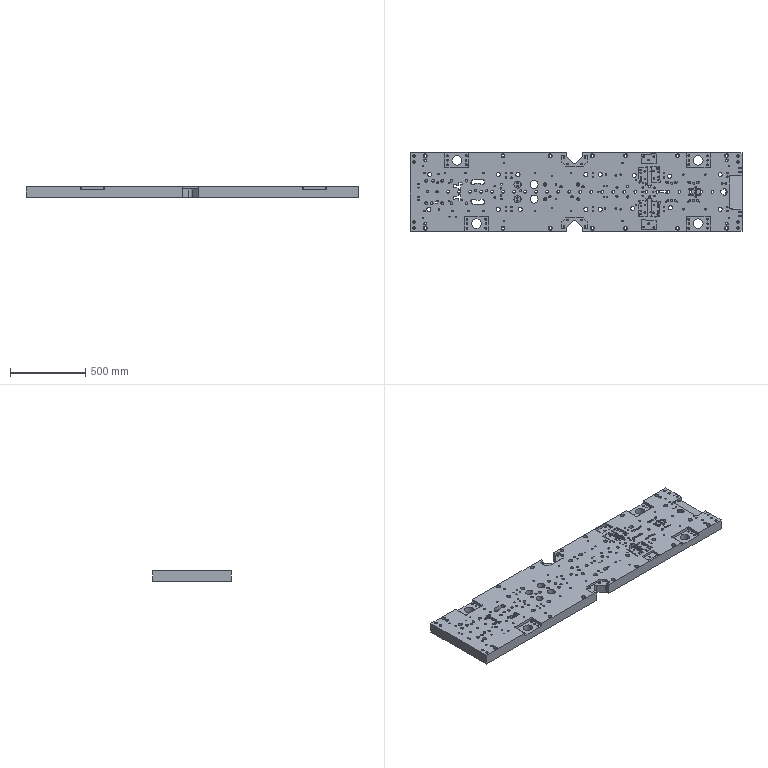Part | NX | features LP-1 2 | 1 solid | 1092 faces | box 2200 x 520 x 70 mm | volume 72651066 mm3 | cylinder 527 | cone 260 | plane 258 | spline 47 | commonest cylinder face diameters 10 x78 8.5 x56 6 x50 18.003 x35 8 x26 18.505 x25